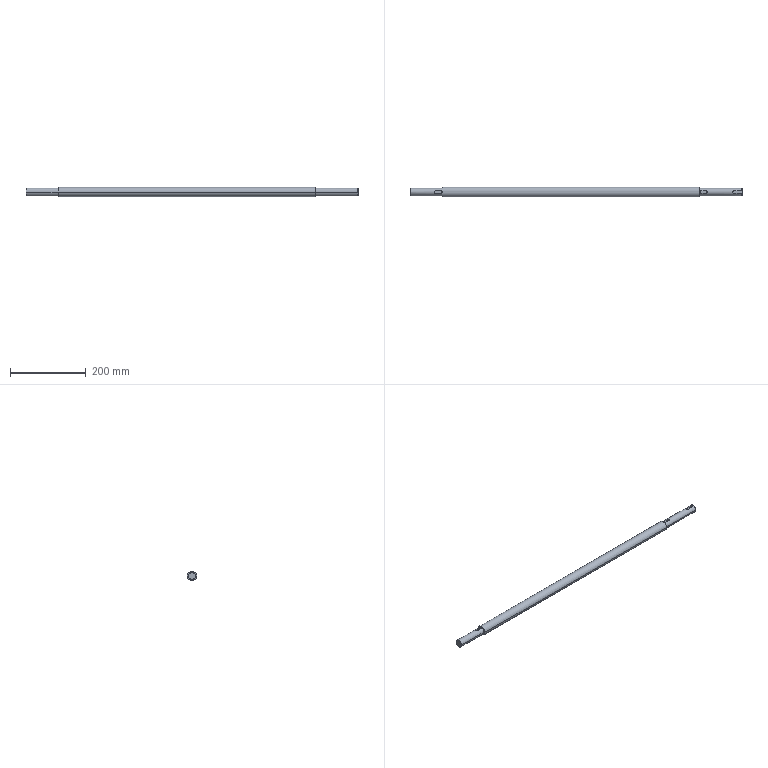Part | STEP file | J011-EBZ05-03-06-Part-1 | 1 solid | 42 faces | box 874 x 25 x 25 mm | volume 391880 mm3 | cylinder 17 | plane 14 | cone 7 | torus 4 | commonest cylinder face diameters 6 x7 20 x4 6.65 x2 8 x2 25 x2
STEP:
#1=CARTESIAN_POINT('',(852.08,0.,0.));
#2=VERTEX_POINT('',#1);
#3=CARTESIAN_POINT('',(854.,3.325,0.));
#4=VERTEX_POINT('',#3);
#5=CARTESIAN_POINT('',(854.,3.325,0.));
#6=DIRECTION('',(0.5,0.866,0.));
#7=VECTOR('',#6,1000.);
#8=LINE('',#5,#7);
#9=EDGE_CURVE('',#2,#4,#8,.T.);
#10=ORIENTED_EDGE('',*,*,#9,.F.);
#11=CARTESIAN_POINT('',(854.,-3.325,0.));
#12=VERTEX_POINT('',#11);
#13=CARTESIAN_POINT('',(854.,-3.325,0.));
#14=DIRECTION('',(0.5,-0.866,0.));
#15=VECTOR('',#14,1000.);
#16=LINE('',#13,#15);
#17=EDGE_CURVE('',#2,#12,#16,.T.);
#18=ORIENTED_EDGE('',*,*,#17,.T.);
#19=CARTESIAN_POINT('',(854.,0.,0.));
#20=DIRECTION('',(1.,0.,0.));
#21=DIRECTION('',(0.,1.,0.));
#22=AXIS2_PLACEMENT_3D('',#19,#20,#21);
#23=CIRCLE('',#22,3.325);
#24=EDGE_CURVE('',#12,#4,#23,.T.);
#25=ORIENTED_EDGE('',*,*,#24,.T.);
#26=EDGE_LOOP('',(#10,#18,#25));
#27=FACE_OUTER_BOUND('',#26,.T.);
#28=CARTESIAN_POINT('',(854.,0.,0.));
#29=DIRECTION('',(1.,0.,0.));
#30=DIRECTION('',(0.,1.,0.));
#31=AXIS2_PLACEMENT_3D('',#28,#29,#30);
#32=CONICAL_SURFACE('',#31,3.325,1.047);
#33=ADVANCED_FACE('',(#27),#32,.F.);
#34=ORIENTED_EDGE('',*,*,#24,.F.);
#35=CARTESIAN_POINT('',(858.,-3.325,0.));
#36=VERTEX_POINT('',#35);
#37=CARTESIAN_POINT('',(874.,-3.325,0.));
#38=DIRECTION('',(1.,0.,0.));
#39=VECTOR('',#38,1000.);
#40=LINE('',#37,#39);
#41=EDGE_CURVE('',#12,#36,#40,.T.);
#42=ORIENTED_EDGE('',*,*,#41,.T.);
#43=CARTESIAN_POINT('',(858.,3.325,0.));
#44=VERTEX_POINT('',#43);
#45=CARTESIAN_POINT('',(858.,0.,0.));
#46=DIRECTION('',(1.,0.,0.));
#47=DIRECTION('',(0.,1.,0.));
#48=AXIS2_PLACEMENT_3D('',#45,#46,#47);
#49=CIRCLE('',#48,3.325);
#50=EDGE_CURVE('',#36,#44,#49,.T.);
#51=ORIENTED_EDGE('',*,*,#50,.T.);
#52=CARTESIAN_POINT('',(874.,3.325,0.));
#53=DIRECTION('',(1.,0.,0.));
#54=VECTOR('',#53,1000.);
#55=LINE('',#52,#54);
#56=EDGE_CURVE('',#4,#44,#55,.T.);
#57=ORIENTED_EDGE('',*,*,#56,.F.);
#58=EDGE_LOOP('',(#34,#42,#51,#57));
#59=FACE_OUTER_BOUND('',#58,.T.);
#60=CARTESIAN_POINT('',(874.,0.,0.));
#61=DIRECTION('',(1.,0.,0.));
#62=DIRECTION('',(0.,1.,0.));
#63=AXIS2_PLACEMENT_3D('',#60,#61,#62);
#64=CYLINDRICAL_SURFACE('',#63,3.325);
#65=ADVANCED_FACE('',(#59),#64,.F.);
#66=CARTESIAN_POINT('',(858.,-4.,0.));
#67=VERTEX_POINT('',#66);
#68=CARTESIAN_POINT('',(858.,4.,0.));
#69=VERTEX_POINT('',#68);
#70=CARTESIAN_POINT('',(858.,0.,0.));
#71=DIRECTION('',(1.,0.,0.));
#72=DIRECTION('',(0.,1.,0.));
#73=AXIS2_PLACEMENT_3D('',#70,#71,#72);
#74=CIRCLE('',#73,4.);
#75=EDGE_CURVE('',#67,#69,#74,.T.);
#76=ORIENTED_EDGE('',*,*,#75,.F.);
#77=CARTESIAN_POINT('',(874.,-4.,0.));
#78=VERTEX_POINT('',#77);
#79=CARTESIAN_POINT('',(874.,-4.,0.));
#80=DIRECTION('',(1.,0.,0.));
#81=VECTOR('',#80,1000.);
#82=LINE('',#79,#81);
#83=EDGE_CURVE('',#67,#78,#82,.T.);
#84=ORIENTED_EDGE('',*,*,#83,.T.);
#85=CARTESIAN_POINT('',(874.,4.,0.));
#86=VERTEX_POINT('',#85);
#87=CARTESIAN_POINT('',(874.,0.,0.));
#88=DIRECTION('',(1.,0.,0.));
#89=DIRECTION('',(0.,1.,0.));
#90=AXIS2_PLACEMENT_3D('',#87,#88,#89);
#91=CIRCLE('',#90,4.);
#92=EDGE_CURVE('',#78,#86,#91,.T.);
#93=ORIENTED_EDGE('',*,*,#92,.T.);
#94=CARTESIAN_POINT('',(874.,4.,0.));
#95=DIRECTION('',(1.,0.,0.));
#96=VECTOR('',#95,1000.);
#97=LINE('',#94,#96);
#98=EDGE_CURVE('',#69,#86,#97,.T.);
#99=ORIENTED_EDGE('',*,*,#98,.F.);
#100=EDGE_LOOP('',(#76,#84,#93,#99));
#101=FACE_OUTER_BOUND('',#100,.T.);
#102=CARTESIAN_POINT('',(874.,0.,0.));
#103=DIRECTION('',(1.,0.,0.));
#104=DIRECTION('',(0.,1.,0.));
#105=AXIS2_PLACEMENT_3D('',#102,#103,#104);
#106=CYLINDRICAL_SURFACE('',#105,4.);
#107=ADVANCED_FACE('',(#101),#106,.F.);
#108=CARTESIAN_POINT('',(762.8,0.,10.));
#109=VERTEX_POINT('',#108);
#110=CARTESIAN_POINT('',(765.8,3.,9.539));
#111=VERTEX_POINT('',#110);
#112=CARTESIAN_POINT('',(762.8,0.,10.));
#113=CARTESIAN_POINT('',(762.8,0.1993,10.));
#114=CARTESIAN_POINT('',(762.82,0.3951,9.994));
#115=CARTESIAN_POINT('',(762.897,0.7799,9.971));
#116=CARTESIAN_POINT('',(762.955,0.971,9.954));
#117=CARTESIAN_POINT('',(763.106,1.334,9.912));
#118=CARTESIAN_POINT('',(763.198,1.505,9.887));
#119=CARTESIAN_POINT('',(763.415,1.831,9.832));
#120=CARTESIAN_POINT('',(763.541,1.984,9.802));
#121=CARTESIAN_POINT('',(763.953,2.396,9.713));
#122=CARTESIAN_POINT('',(764.286,2.619,9.652));
#123=CARTESIAN_POINT('',(764.826,2.844,9.587));
#124=CARTESIAN_POINT('',(765.016,2.902,9.57));
#125=CARTESIAN_POINT('',(765.404,2.98,9.546));
#126=CARTESIAN_POINT('',(765.601,3.,9.539));
#127=CARTESIAN_POINT('',(765.8,3.,9.539));
#128=B_SPLINE_CURVE_WITH_KNOTS('',3,(#112,#113,#114,#115,#116,#117,#118,#119,#120,#121,#122,#123,#124,#125,#126,#127),.UNSPECIFIED.,.F.,.F.,(4,2,2,2,2,2,2,4),(0.,0.0005892,0.001178,0.001768,0.002357,0.003535,0.004125,0.004714),.UNSPECIFIED.);
#129=EDGE_CURVE('',#109,#111,#128,.T.);
#130=ORIENTED_EDGE('',*,*,#129,.F.);
#131=CARTESIAN_POINT('',(762.8,0.,6.5));
#132=VERTEX_POINT('',#131);
#133=CARTESIAN_POINT('',(762.8,0.,10.52));
#134=DIRECTION('',(0.,0.,-1.));
#135=VECTOR('',#134,1000.);
#136=LINE('',#133,#135);
#137=EDGE_CURVE('',#109,#132,#136,.T.);
#138=ORIENTED_EDGE('',*,*,#137,.T.);
#139=CARTESIAN_POINT('',(765.8,3.,6.5));
#140=VERTEX_POINT('',#139);
#141=CARTESIAN_POINT('',(765.8,0.,6.5));
#142=DIRECTION('',(0.,0.,1.));
#143=DIRECTION('',(-1.,0.,0.));
#144=AXIS2_PLACEMENT_3D('',#141,#142,#143);
#145=CIRCLE('',#144,3.);
#146=EDGE_CURVE('',#140,#132,#145,.T.);
#147=ORIENTED_EDGE('',*,*,#146,.F.);
#148=CARTESIAN_POINT('',(765.8,3.,6.5));
#149=DIRECTION('',(0.,0.,-1.));
#150=VECTOR('',#149,1000.);
#151=LINE('',#148,#150);
#152=EDGE_CURVE('',#111,#140,#151,.T.);
#153=ORIENTED_EDGE('',*,*,#152,.F.);
#154=EDGE_LOOP('',(#130,#138,#147,#153));
#155=FACE_OUTER_BOUND('',#154,.T.);
#156=CARTESIAN_POINT('',(765.8,0.,10.52));
#157=DIRECTION('',(0.,0.,-1.));
#158=DIRECTION('',(-1.,0.,0.));
#159=AXIS2_PLACEMENT_3D('',#156,#157,#158);
#160=CYLINDRICAL_SURFACE('',#159,3.);
#161=ADVANCED_FACE('',(#155),#160,.F.);
#162=CARTESIAN_POINT('',(64.15,0.,10.));
#163=VERTEX_POINT('',#162);
#164=CARTESIAN_POINT('',(67.15,3.,9.539));
#165=VERTEX_POINT('',#164);
#166=CARTESIAN_POINT('',(64.15,0.,10.));
#167=CARTESIAN_POINT('',(64.15,0.1968,10.));
#168=CARTESIAN_POINT('',(64.17,0.3967,9.994));
#169=CARTESIAN_POINT('',(64.247,0.7821,9.971));
#170=CARTESIAN_POINT('',(64.304,0.9695,9.955));
#171=CARTESIAN_POINT('',(64.456,1.334,9.912));
#172=CARTESIAN_POINT('',(64.549,1.507,9.887));
#173=CARTESIAN_POINT('',(64.766,1.831,9.832));
#174=CARTESIAN_POINT('',(64.891,1.983,9.802));
#175=CARTESIAN_POINT('',(65.167,2.26,9.742));
#176=CARTESIAN_POINT('',(65.317,2.383,9.713));
#177=CARTESIAN_POINT('',(65.641,2.6,9.657));
#178=CARTESIAN_POINT('',(65.817,2.694,9.63));
#179=CARTESIAN_POINT('',(66.178,2.845,9.587));
#180=CARTESIAN_POINT('',(66.365,2.902,9.57));
#181=CARTESIAN_POINT('',(66.751,2.98,9.546));
#182=CARTESIAN_POINT('',(66.951,3.,9.539));
#183=CARTESIAN_POINT('',(67.15,3.,9.539));
#184=B_SPLINE_CURVE_WITH_KNOTS('',3,(#166,#167,#168,#169,#170,#171,#172,#173,#174,#175,#176,#177,#178,#179,#180,#181,#182,#183),.UNSPECIFIED.,.F.,.F.,(4,2,2,2,2,2,2,2,4),(0.004718,0.005307,0.005896,0.006485,0.007074,0.007663,0.008252,0.008842,0.009431),.UNSPECIFIED.);
#185=EDGE_CURVE('',#163,#165,#184,.T.);
#186=ORIENTED_EDGE('',*,*,#185,.F.);
#187=CARTESIAN_POINT('',(64.15,0.,6.5));
#188=VERTEX_POINT('',#187);
#189=CARTESIAN_POINT('',(64.15,0.,10.));
#190=DIRECTION('',(0.,0.,-1.));
#191=VECTOR('',#190,1000.);
#192=LINE('',#189,#191);
#193=EDGE_CURVE('',#163,#188,#192,.T.);
#194=ORIENTED_EDGE('',*,*,#193,.T.);
#195=CARTESIAN_POINT('',(67.15,3.,6.5));
#196=VERTEX_POINT('',#195);
#197=CARTESIAN_POINT('',(67.15,0.,6.5));
#198=DIRECTION('',(0.,0.,1.));
#199=DIRECTION('',(1.,0.,0.));
#200=AXIS2_PLACEMENT_3D('',#197,#198,#199);
#201=CIRCLE('',#200,3.);
#202=EDGE_CURVE('',#196,#188,#201,.T.);
#203=ORIENTED_EDGE('',*,*,#202,.F.);
#204=CARTESIAN_POINT('',(67.15,3.,10.));
#205=DIRECTION('',(0.,0.,-1.));
#206=VECTOR('',#205,1000.);
#207=LINE('',#204,#206);
#208=EDGE_CURVE('',#165,#196,#207,.T.);
#209=ORIENTED_EDGE('',*,*,#208,.F.);
#210=EDGE_LOOP('',(#186,#194,#203,#209));
#211=FACE_OUTER_BOUND('',#210,.T.);
#212=CARTESIAN_POINT('',(67.15,0.,10.));
#213=DIRECTION('',(0.,0.,-1.));
#214=DIRECTION('',(-1.,0.,0.));
#215=AXIS2_PLACEMENT_3D('',#212,#213,#214);
#216=CYLINDRICAL_SURFACE('',#215,3.);
#217=ADVANCED_FACE('',(#211),#216,.F.);
#218=CARTESIAN_POINT('',(762.3,10.,0.));
#219=VERTEX_POINT('',#218);
#220=CARTESIAN_POINT('',(762.3,-10.,0.));
#221=VERTEX_POINT('',#220);
#222=CARTESIAN_POINT('',(762.3,0.,0.));
#223=DIRECTION('',(1.,0.,0.));
#224=DIRECTION('',(0.,-1.,0.));
#225=AXIS2_PLACEMENT_3D('',#222,#223,#224);
#226=CIRCLE('',#225,10.);
#227=EDGE_CURVE('',#219,#221,#226,.T.);
#228=ORIENTED_EDGE('',*,*,#227,.F.);
#229=CARTESIAN_POINT('',(761.8,10.5,0.));
#230=VERTEX_POINT('',#229);
#231=CARTESIAN_POINT('',(762.3,10.5,0.));
#232=DIRECTION('',(0.,0.,-1.));
#233=DIRECTION('',(0.,1.,0.));
#234=AXIS2_PLACEMENT_3D('',#231,#232,#233);
#235=CIRCLE('',#234,0.5);
#236=EDGE_CURVE('',#219,#230,#235,.T.);
#237=ORIENTED_EDGE('',*,*,#236,.T.);
#238=CARTESIAN_POINT('',(761.8,-10.5,0.));
#239=VERTEX_POINT('',#238);
#240=CARTESIAN_POINT('',(761.8,0.,0.));
#241=DIRECTION('',(-1.,0.,0.));
#242=DIRECTION('',(0.,-1.,0.));
#243=AXIS2_PLACEMENT_3D('',#240,#241,#242);
#244=CIRCLE('',#243,10.5);
#245=EDGE_CURVE('',#239,#230,#244,.T.);
#246=ORIENTED_EDGE('',*,*,#245,.F.);
#247=CARTESIAN_POINT('',(762.3,-10.5,0.));
#248=DIRECTION('',(0.,0.,1.));
#249=DIRECTION('',(1.,0.,0.));
#250=AXIS2_PLACEMENT_3D('',#247,#248,#249);
#251=CIRCLE('',#250,0.5);
#252=EDGE_CURVE('',#221,#239,#251,.T.);
#253=ORIENTED_EDGE('',*,*,#252,.F.);
#254=EDGE_LOOP('',(#228,#237,#246,#253));
#255=FACE_OUTER_BOUND('',#254,.T.);
#256=CARTESIAN_POINT('',(762.3,0.,0.));
#257=DIRECTION('',(1.,0.,0.));
#258=DIRECTION('',(0.,-1.,0.));
#259=AXIS2_PLACEMENT_3D('',#256,#257,#258);
#260=TOROIDAL_SURFACE('',#259,10.5,0.5);
#261=ADVANCED_FACE('',(#255),#260,.F.);
#262=CARTESIAN_POINT('',(84.7,-10.,0.));
#263=VERTEX_POINT('',#262);
#264=CARTESIAN_POINT('',(84.7,10.,0.));
#265=VERTEX_POINT('',#264);
#266=CARTESIAN_POINT('',(84.7,0.,0.));
#267=DIRECTION('',(-1.,0.,0.));
#268=DIRECTION('',(0.,1.,0.));
#269=AXIS2_PLACEMENT_3D('',#266,#267,#268);
#270=CIRCLE('',#269,10.);
#271=EDGE_CURVE('',#263,#265,#270,.T.);
#272=ORIENTED_EDGE('',*,*,#271,.F.);
#273=CARTESIAN_POINT('',(85.2,-10.5,0.));
#274=VERTEX_POINT('',#273);
#275=CARTESIAN_POINT('',(84.7,-10.5,0.));
#276=DIRECTION('',(0.,0.,-1.));
#277=DIRECTION('',(0.,1.,0.));
#278=AXIS2_PLACEMENT_3D('',#275,#276,#277);
#279=CIRCLE('',#278,0.5);
#280=EDGE_CURVE('',#263,#274,#279,.T.);
#281=ORIENTED_EDGE('',*,*,#280,.T.);
#282=CARTESIAN_POINT('',(85.2,10.5,0.));
#283=VERTEX_POINT('',#282);
#284=CARTESIAN_POINT('',(85.2,0.,0.));
#285=DIRECTION('',(1.,0.,0.));
#286=DIRECTION('',(0.,1.,0.));
#287=AXIS2_PLACEMENT_3D('',#284,#285,#286);
#288=CIRCLE('',#287,10.5);
#289=EDGE_CURVE('',#283,#274,#288,.T.);
#290=ORIENTED_EDGE('',*,*,#289,.F.);
#291=CARTESIAN_POINT('',(84.7,10.5,0.));
#292=DIRECTION('',(0.,0.,1.));
#293=DIRECTION('',(1.,0.,0.));
#294=AXIS2_PLACEMENT_3D('',#291,#292,#293);
#295=CIRCLE('',#294,0.5);
#296=EDGE_CURVE('',#265,#283,#295,.T.);
#297=ORIENTED_EDGE('',*,*,#296,.F.);
#298=EDGE_LOOP('',(#272,#281,#290,#297));
#299=FACE_OUTER_BOUND('',#298,.T.);
#300=CARTESIAN_POINT('',(84.7,0.,0.));
#301=DIRECTION('',(-1.,0.,0.));
#302=DIRECTION('',(0.,1.,0.));
#303=AXIS2_PLACEMENT_3D('',#300,#301,#302);
#304=TOROIDAL_SURFACE('',#303,10.5,0.5);
#305=ADVANCED_FACE('',(#299),#304,.F.);
#306=CARTESIAN_POINT('',(0.,-9.,0.));
#307=VERTEX_POINT('',#306);
#308=CARTESIAN_POINT('',(0.,9.,0.));
#309=VERTEX_POINT('',#308);
#310=CARTESIAN_POINT('',(0.,0.,0.));
#311=DIRECTION('',(1.,0.,0.));
#312=DIRECTION('',(0.,-1.,0.));
#313=AXIS2_PLACEMENT_3D('',#310,#311,#312);
#314=CIRCLE('',#313,9.);
#315=EDGE_CURVE('',#307,#309,#314,.T.);
#316=ORIENTED_EDGE('',*,*,#315,.T.);
#317=CARTESIAN_POINT('',(1.,10.,0.));
#318=VERTEX_POINT('',#317);
#319=CARTESIAN_POINT('',(1.,10.,0.));
#320=DIRECTION('',(0.7071,0.7071,0.));
#321=VECTOR('',#320,1000.);
#322=LINE('',#319,#321);
#323=EDGE_CURVE('',#309,#318,#322,.T.);
#324=ORIENTED_EDGE('',*,*,#323,.T.);
#325=CARTESIAN_POINT('',(1.,-10.,0.));
#326=VERTEX_POINT('',#325);
#327=CARTESIAN_POINT('',(1.,0.,0.));
#328=DIRECTION('',(1.,0.,0.));
#329=DIRECTION('',(0.,-1.,0.));
#330=AXIS2_PLACEMENT_3D('',#327,#328,#329);
#331=CIRCLE('',#330,10.);
#332=EDGE_CURVE('',#326,#318,#331,.T.);
#333=ORIENTED_EDGE('',*,*,#332,.F.);
#334=CARTESIAN_POINT('',(1.,-10.,0.));
#335=DIRECTION('',(0.7071,-0.7071,0.));
#336=VECTOR('',#335,1000.);
#337=LINE('',#334,#336);
#338=EDGE_CURVE('',#307,#326,#337,.T.);
#339=ORIENTED_EDGE('',*,*,#338,.F.);
#340=EDGE_LOOP('',(#316,#324,#333,#339));
#341=FACE_OUTER_BOUND('',#340,.T.);
#342=CARTESIAN_POINT('',(1.,0.,0.));
#343=DIRECTION('',(1.,0.,0.));
#344=DIRECTION('',(0.,-1.,0.));
#345=AXIS2_PLACEMENT_3D('',#342,#343,#344);
#346=CONICAL_SURFACE('',#345,10.,0.7854);
#347=ADVANCED_FACE('',(#341),#346,.T.);
#348=CARTESIAN_POINT('',(85.2,-12.5,0.));
#349=VERTEX_POINT('',#348);
#350=CARTESIAN_POINT('',(85.2,12.5,0.));
#351=VERTEX_POINT('',#350);
#352=CARTESIAN_POINT('',(85.2,0.,0.));
#353=DIRECTION('',(1.,0.,0.));
#354=DIRECTION('',(0.,-1.,0.));
#355=AXIS2_PLACEMENT_3D('',#352,#353,#354);
#356=CIRCLE('',#355,12.5);
#357=EDGE_CURVE('',#349,#351,#356,.T.);
#358=ORIENTED_EDGE('',*,*,#357,.T.);
#359=CARTESIAN_POINT('',(761.8,12.5,0.));
#360=VERTEX_POINT('',#359);
#361=CARTESIAN_POINT('',(154.523,12.5,0.));
#362=DIRECTION('',(1.,0.,0.));
#363=VECTOR('',#362,1000.);
#364=LINE('',#361,#363);
#365=EDGE_CURVE('',#351,#360,#364,.T.);
#366=ORIENTED_EDGE('',*,*,#365,.T.);
#367=CARTESIAN_POINT('',(761.8,-12.5,0.));
#368=VERTEX_POINT('',#367);
#369=CARTESIAN_POINT('',(761.8,0.,0.));
#370=DIRECTION('',(1.,0.,0.));
#371=DIRECTION('',(0.,-1.,0.));
#372=AXIS2_PLACEMENT_3D('',#369,#370,#371);
#373=CIRCLE('',#372,12.5);
#374=EDGE_CURVE('',#368,#360,#373,.T.);
#375=ORIENTED_EDGE('',*,*,#374,.F.);
#376=CARTESIAN_POINT('',(154.523,-12.5,0.));
#377=DIRECTION('',(1.,0.,0.));
#378=VECTOR('',#377,1000.);
#379=LINE('',#376,#378);
#380=EDGE_CURVE('',#349,#368,#379,.T.);
#381=ORIENTED_EDGE('',*,*,#380,.F.);
#382=EDGE_LOOP('',(#358,#366,#375,#381));
#383=FACE_OUTER_BOUND('',#382,.T.);
#384=CARTESIAN_POINT('',(154.523,0.,0.));
#385=DIRECTION('',(1.,0.,0.));
#386=DIRECTION('',(0.,-1.,0.));
#387=AXIS2_PLACEMENT_3D('',#384,#385,#386);
#388=CYLINDRICAL_SURFACE('',#387,12.5);
#389=ADVANCED_FACE('',(#383),#388,.T.);
#390=CARTESIAN_POINT('',(762.3,0.,0.));
#391=DIRECTION('',(1.,0.,0.));
#392=DIRECTION('',(0.,-1.,0.));
#393=AXIS2_PLACEMENT_3D('',#390,#391,#392);
#394=CIRCLE('',#393,10.);
#395=EDGE_CURVE('',#221,#219,#394,.T.);
#396=ORIENTED_EDGE('',*,*,#395,.T.);
#397=CARTESIAN_POINT('',(873.,10.,0.));
#398=VERTEX_POINT('',#397);
#399=CARTESIAN_POINT('',(154.523,10.,0.));
#400=DIRECTION('',(1.,0.,0.));
#401=VECTOR('',#400,1000.);
#402=LINE('',#399,#401);
#403=EDGE_CURVE('',#219,#398,#402,.T.);
#404=ORIENTED_EDGE('',*,*,#403,.T.);
#405=CARTESIAN_POINT('',(873.,-10.,0.));
#406=VERTEX_POINT('',#405);
#407=CARTESIAN_POINT('',(873.,0.,0.));
#408=DIRECTION('',(1.,0.,0.));
#409=DIRECTION('',(0.,-1.,0.));
#410=AXIS2_PLACEMENT_3D('',#407,#408,#409);
#411=CIRCLE('',#410,10.);
#412=EDGE_CURVE('',#406,#398,#411,.T.);
#413=ORIENTED_EDGE('',*,*,#412,.F.);
#414=CARTESIAN_POINT('',(154.523,-10.,0.));
#415=DIRECTION('',(1.,0.,0.));
#416=VECTOR('',#415,1000.);
#417=LINE('',#414,#416);
#418=EDGE_CURVE('',#221,#406,#417,.T.);
#419=ORIENTED_EDGE('',*,*,#418,.F.);
#420=EDGE_LOOP('',(#396,#404,#413,#419));
#421=FACE_OUTER_BOUND('',#420,.T.);
#422=CARTESIAN_POINT('',(154.523,0.,0.));
#423=DIRECTION('',(1.,0.,0.));
#424=DIRECTION('',(0.,-1.,0.));
#425=AXIS2_PLACEMENT_3D('',#422,#423,#424);
#426=CYLINDRICAL_SURFACE('',#425,10.);
#427=ADVANCED_FACE('',(#421),#426,.T.);
#428=CARTESIAN_POINT('',(874.,-9.,0.));
#429=VERTEX_POINT('',#428);
#430=CARTESIAN_POINT('',(874.,9.,0.));
#431=VERTEX_POINT('',#430);
#432=CARTESIAN_POINT('',(874.,0.,0.));
#433=DIRECTION('',(1.,0.,0.));
#434=DIRECTION('',(0.,-1.,0.));
#435=AXIS2_PLACEMENT_3D('',#432,#433,#434);
#436=CIRCLE('',#435,9.);
#437=EDGE_CURVE('',#429,#431,#436,.T.);
#438=ORIENTED_EDGE('',*,*,#437,.F.);
#439=CARTESIAN_POINT('',(874.,-9.,0.));
#440=DIRECTION('',(-0.7071,-0.7071,0.));
#441=VECTOR('',#440,1000.);
#442=LINE('',#439,#441);
#443=EDGE_CURVE('',#429,#406,#442,.T.);
#444=ORIENTED_EDGE('',*,*,#443,.T.);
#445=ORIENTED_EDGE('',*,*,#412,.T.);
#446=CARTESIAN_POINT('',(874.,9.,0.));
#447=DIRECTION('',(-0.7071,0.7071,0.));
#448=VECTOR('',#447,1000.);
#449=LINE('',#446,#448);
#450=EDGE_CURVE('',#431,#398,#449,.T.);
#451=ORIENTED_EDGE('',*,*,#450,.F.);
#452=EDGE_LOOP('',(#438,#444,#445,#451));
#453=FACE_OUTER_BOUND('',#452,.T.);
#454=CARTESIAN_POINT('',(874.,0.,0.));
#455=DIRECTION('',(-1.,0.,0.));
#456=DIRECTION('',(0.,1.,0.));
#457=AXIS2_PLACEMENT_3D('',#454,#455,#456);
#458=CONICAL_SURFACE('',#457,9.,0.7854);
#459=ADVANCED_FACE('',(#453),#458,.T.);
#460=CARTESIAN_POINT('',(874.,3.,8.485));
#461=VERTEX_POINT('',#460);
#462=CARTESIAN_POINT('',(874.,0.,0.));
#463=DIRECTION('',(1.,0.,0.));
#464=DIRECTION('',(0.,-1.,0.));
#465=AXIS2_PLACEMENT_3D('',#462,#463,#464);
#466=CIRCLE('',#465,9.);
#467=EDGE_CURVE('',#431,#461,#466,.T.);
#468=ORIENTED_EDGE('',*,*,#467,.F.);
#469=ORIENTED_EDGE('',*,*,#450,.T.);
#470=CARTESIAN_POINT('',(873.,3.,9.539));
#471=VERTEX_POINT('',#470);
#472=CARTESIAN_POINT('',(873.,0.,0.));
#473=DIRECTION('',(1.,0.,0.));
#474=DIRECTION('',(0.,-1.,0.));
#475=AXIS2_PLACEMENT_3D('',#472,#473,#474);
#476=CIRCLE('',#475,10.);
#477=EDGE_CURVE('',#398,#471,#476,.T.);
#478=ORIENTED_EDGE('',*,*,#477,.T.);
#479=CARTESIAN_POINT('',(874.,3.,8.485));
#480=CARTESIAN_POINT('',(873.668,3.,8.838));
#481=CARTESIAN_POINT('',(873.334,3.,9.189));
#482=CARTESIAN_POINT('',(873.,3.,9.539));
#483=B_SPLINE_CURVE_WITH_KNOTS('',3,(#479,#480,#481,#482),.UNSPECIFIED.,.F.,.F.,(4,4),(0.005441,0.006894),.UNSPECIFIED.);
#484=EDGE_CURVE('',#461,#471,#483,.T.);
#485=ORIENTED_EDGE('',*,*,#484,.F.);
#486=EDGE_LOOP('',(#468,#469,#478,#485));
#487=FACE_OUTER_BOUND('',#486,.T.);
#488=CARTESIAN_POINT('',(874.,0.,0.));
#489=DIRECTION('',(-1.,0.,0.));
#490=DIRECTION('',(0.,1.,0.));
#491=AXIS2_PLACEMENT_3D('',#488,#489,#490);
#492=CONICAL_SURFACE('',#491,9.,0.7854);
#493=ADVANCED_FACE('',(#487),#492,.T.);
#494=ORIENTED_EDGE('',*,*,#332,.T.);
#495=CARTESIAN_POINT('',(154.523,10.,0.));
#496=DIRECTION('',(1.,0.,0.));
#497=VECTOR('',#496,1000.);
#498=LINE('',#495,#497);
#499=EDGE_CURVE('',#318,#265,#498,.T.);
#500=ORIENTED_EDGE('',*,*,#499,.T.);
#501=CARTESIAN_POINT('',(84.7,0.,0.));
#502=DIRECTION('',(-1.,0.,0.));
#503=DIRECTION('',(0.,1.,0.));
#504=AXIS2_PLACEMENT_3D('',#501,#502,#503);
#505=CIRCLE('',#504,10.);
#506=EDGE_CURVE('',#265,#263,#505,.T.);
#507=ORIENTED_EDGE('',*,*,#506,.T.);
#508=CARTESIAN_POINT('',(154.523,-10.,0.));
#509=DIRECTION('',(1.,0.,0.));
#510=VECTOR('',#509,1000.);
#511=LINE('',#508,#510);
#512=EDGE_CURVE('',#326,#263,#511,.T.);
#513=ORIENTED_EDGE('',*,*,#512,.F.);
#514=EDGE_LOOP('',(#494,#500,#507,#513));
#515=FACE_OUTER_BOUND('',#514,.T.);
#516=CARTESIAN_POINT('',(154.523,0.,0.));
#517=DIRECTION('',(1.,0.,0.));
#518=DIRECTION('',(0.,-1.,0.));
#519=AXIS2_PLACEMENT_3D('',#516,#517,#518);
#520=CYLINDRICAL_SURFACE('',#519,10.);
#521=ADVANCED_FACE('',(#515),#520,.T.);
#522=CARTESIAN_POINT('',(874.,0.,0.));
#523=DIRECTION('',(1.,0.,0.));
#524=DIRECTION('',(0.,1.,0.));
#525=AXIS2_PLACEMENT_3D('',#522,#523,#524);
#526=CIRCLE('',#525,4.);
#527=EDGE_CURVE('',#86,#78,#526,.T.);
#528=ORIENTED_EDGE('',*,*,#527,.F.);
#529=ORIENTED_EDGE('',*,*,#92,.F.);
#530=EDGE_LOOP('',(#528,#529));
#531=FACE_BOUND('',#530,.T.);
#532=CARTESIAN_POINT('',(874.,3.,6.5));
#533=VERTEX_POINT('',#532);
#534=CARTESIAN_POINT('',(874.,-3.,6.5));
#535=VERTEX_POINT('',#534);
#536=CARTESIAN_POINT('',(874.,0.,6.5));
#537=DIRECTION('',(0.,-1.,0.));
#538=VECTOR('',#537,1000.);
#539=LINE('',#536,#538);
#540=EDGE_CURVE('',#533,#535,#539,.T.);
#541=ORIENTED_EDGE('',*,*,#540,.T.);
#542=CARTESIAN_POINT('',(874.,-3.,8.485));
#543=VERTEX_POINT('',#542);
#544=CARTESIAN_POINT('',(874.,-3.,10.52));
#545=DIRECTION('',(0.,0.,1.));
#546=VECTOR('',#545,1000.);
#547=LINE('',#544,#546);
#548=EDGE_CURVE('',#535,#543,#547,.T.);
#549=ORIENTED_EDGE('',*,*,#548,.T.);
#550=CARTESIAN_POINT('',(874.,0.,0.));
#551=DIRECTION('',(1.,0.,0.));
#552=DIRECTION('',(0.,-1.,0.));
#553=AXIS2_PLACEMENT_3D('',#550,#551,#552);
#554=CIRCLE('',#553,9.);
#555=EDGE_CURVE('',#543,#429,#554,.T.);
#556=ORIENTED_EDGE('',*,*,#555,.T.);
#557=ORIENTED_EDGE('',*,*,#437,.T.);
#558=ORIENTED_EDGE('',*,*,#467,.T.);
#559=CARTESIAN_POINT('',(874.,3.,10.52));
#560=DIRECTION('',(0.,0.,-1.));
#561=VECTOR('',#560,1000.);
#562=LINE('',#559,#561);
#563=EDGE_CURVE('',#461,#533,#562,.T.);
#564=ORIENTED_EDGE('',*,*,#563,.T.);
#565=EDGE_LOOP('',(#541,#549,#556,#557,#558,#564));
#566=FACE_OUTER_BOUND('',#565,.T.);
#567=CARTESIAN_POINT('',(874.,0.,0.));
#568=DIRECTION('',(1.,0.,0.));
#569=DIRECTION('',(0.,-1.,0.));
#570=AXIS2_PLACEMENT_3D('',#567,#568,#569);
#571=PLANE('',#570);
#572=ADVANCED_FACE('',(#531,#566),#571,.T.);
#573=ORIENTED_EDGE('',*,*,#499,.F.);
#574=CARTESIAN_POINT('',(1.,0.,0.));
#575=DIRECTION('',(1.,0.,0.));
#576=DIRECTION('',(0.,-1.,0.));
#577=AXIS2_PLACEMENT_3D('',#574,#575,#576);
#578=CIRCLE('',#577,10.);
#579=EDGE_CURVE('',#318,#326,#578,.T.);
#580=ORIENTED_EDGE('',*,*,#579,.T.);
#581=ORIENTED_EDGE('',*,*,#512,.T.);
#582=ORIENTED_EDGE('',*,*,#271,.T.);
#583=EDGE_LOOP('',(#573,#580,#581,#582));
#584=FACE_OUTER_BOUND('',#583,.T.);
#585=CARTESIAN_POINT('',(81.15,3.,9.539));
#586=VERTEX_POINT('',#585);
#587=CARTESIAN_POINT('',(154.523,3.,9.539));
#588=DIRECTION('',(1.,0.,0.));
#589=VECTOR('',#588,1000.);
#590=LINE('',#587,#589);
#591=EDGE_CURVE('',#165,#586,#590,.T.);
#592=ORIENTED_EDGE('',*,*,#591,.T.);
#593=CARTESIAN_POINT('',(81.15,-3.,9.539));
#594=VERTEX_POINT('',#593);
#595=CARTESIAN_POINT('',(81.15,3.,9.539));
#596=CARTESIAN_POINT('',(81.349,3.,9.539));
#597=CARTESIAN_POINT('',(81.545,2.98,9.546));
#598=CARTESIAN_POINT('',(81.93,2.903,9.569));
#599=CARTESIAN_POINT('',(82.121,2.845,9.587));
#600=CARTESIAN_POINT('',(82.484,2.694,9.631));
#601=CARTESIAN_POINT('',(82.656,2.602,9.656));
#602=CARTESIAN_POINT('',(82.981,2.385,9.712));
#603=CARTESIAN_POINT('',(83.134,2.259,9.743));
#604=CARTESIAN_POINT('',(83.546,1.847,9.832));
#605=CARTESIAN_POINT('',(83.769,1.514,9.891));
#606=CARTESIAN_POINT('',(83.994,0.9732,9.954));
#607=CARTESIAN_POINT('',(84.053,0.783,9.971));
#608=CARTESIAN_POINT('',(84.13,0.3953,9.994));
#609=CARTESIAN_POINT('',(84.15,0.1999,10.));
#610=CARTESIAN_POINT('',(84.15,-0.194,10.));
#611=CARTESIAN_POINT('',(84.131,-0.394,9.994));
#612=CARTESIAN_POINT('',(84.054,-0.7797,9.971));
#613=CARTESIAN_POINT('',(83.997,-0.9673,9.955));
#614=CARTESIAN_POINT('',(83.845,-1.332,9.913));
#615=CARTESIAN_POINT('',(83.752,-1.506,9.887));
#616=CARTESIAN_POINT('',(83.536,-1.83,9.833));
#617=CARTESIAN_POINT('',(83.41,-1.982,9.803));
#618=CARTESIAN_POINT('',(83.134,-2.259,9.743));
#619=CARTESIAN_POINT('',(82.983,-2.383,9.713));
#620=CARTESIAN_POINT('',(82.66,-2.6,9.657));
#621=CARTESIAN_POINT('',(82.484,-2.694,9.631));
#622=CARTESIAN_POINT('',(82.123,-2.845,9.587));
#623=CARTESIAN_POINT('',(81.936,-2.902,9.57));
#624=CARTESIAN_POINT('',(81.549,-2.98,9.546));
#625=CARTESIAN_POINT('',(81.349,-3.,9.539));
#626=CARTESIAN_POINT('',(81.15,-3.,9.539));
#627=B_SPLINE_CURVE_WITH_KNOTS('',3,(#595,#596,#597,#598,#599,#600,#601,#602,#603,#604,#605,#606,#607,#608,#609,#610,#611,#612,#613,#614,#615,#616,#617,#618,#619,#620,#621,#622,#623,#624,#625,#626),.UNSPECIFIED.,.F.,.F.,(4,2,2,2,2,2,2,2,2,2,2,2,2,2,2,4),(0.,0.0005894,0.001179,0.001768,0.002358,0.003536,0.004126,0.004715,0.005305,0.005894,0.006484,0.007073,0.007662,0.008252,0.008841,0.009431),.UNSPECIFIED.);
#628=EDGE_CURVE('',#586,#594,#627,.T.);
#629=ORIENTED_EDGE('',*,*,#628,.T.);
#630=CARTESIAN_POINT('',(67.15,-3.,9.539));
#631=VERTEX_POINT('',#630);
#632=CARTESIAN_POINT('',(154.523,-3.,9.539));
#633=DIRECTION('',(-1.,0.,0.));
#634=VECTOR('',#633,1000.);
#635=LINE('',#632,#634);
#636=EDGE_CURVE('',#594,#631,#635,.T.);
#637=ORIENTED_EDGE('',*,*,#636,.T.);
#638=CARTESIAN_POINT('',(67.15,-3.,9.539));
#639=CARTESIAN_POINT('',(66.95,-3.,9.539));
#640=CARTESIAN_POINT('',(66.755,-2.98,9.546));
#641=CARTESIAN_POINT('',(66.369,-2.903,9.569));
#642=CARTESIAN_POINT('',(66.178,-2.845,9.587));
#643=CARTESIAN_POINT('',(65.815,-2.694,9.631));
#644=CARTESIAN_POINT('',(65.644,-2.602,9.656));
#645=CARTESIAN_POINT('',(65.318,-2.384,9.712));
#646=CARTESIAN_POINT('',(65.165,-2.258,9.743));
#647=CARTESIAN_POINT('',(64.753,-1.845,9.832));
#648=CARTESIAN_POINT('',(64.53,-1.512,9.892));
#649=CARTESIAN_POINT('',(64.305,-0.971,9.954));
#650=CARTESIAN_POINT('',(64.247,-0.7806,9.971));
#651=CARTESIAN_POINT('',(64.169,-0.3926,9.994));
#652=CARTESIAN_POINT('',(64.15,-0.197,10.));
#653=CARTESIAN_POINT('',(64.15,0.,10.));
#654=B_SPLINE_CURVE_WITH_KNOTS('',3,(#638,#639,#640,#641,#642,#643,#644,#645,#646,#647,#648,#649,#650,#651,#652,#653),.UNSPECIFIED.,.F.,.F.,(4,2,2,2,2,2,2,4),(0.,0.0005898,0.00118,0.001769,0.002359,0.003539,0.004128,0.004718),.UNSPECIFIED.);
#655=EDGE_CURVE('',#631,#163,#654,.T.);
#656=ORIENTED_EDGE('',*,*,#655,.T.);
#657=ORIENTED_EDGE('',*,*,#185,.T.);
#658=EDGE_LOOP('',(#592,#629,#637,#656,#657));
#659=FACE_BOUND('',#658,.T.);
#660=CARTESIAN_POINT('',(154.523,0.,0.));
#661=DIRECTION('',(1.,0.,0.));
#662=DIRECTION('',(0.,-1.,0.));
#663=AXIS2_PLACEMENT_3D('',#660,#661,#662);
#664=CYLINDRICAL_SURFACE('',#663,10.);
#665=ADVANCED_FACE('',(#584,#659),#664,.T.);
#666=ORIENTED_EDGE('',*,*,#443,.F.);
#667=ORIENTED_EDGE('',*,*,#555,.F.);
#668=CARTESIAN_POINT('',(873.,-3.,9.539));
#669=VERTEX_POINT('',#668);
#670=CARTESIAN_POINT('',(873.,-3.,9.539));
#671=CARTESIAN_POINT('',(873.334,-3.,9.189));
#672=CARTESIAN_POINT('',(873.668,-3.,8.838));
#673=CARTESIAN_POINT('',(874.,-3.,8.485));
#674=B_SPLINE_CURVE_WITH_KNOTS('',3,(#670,#671,#672,#673),.UNSPECIFIED.,.F.,.F.,(4,4),(0.005238,0.006691),.UNSPECIFIED.);
#675=EDGE_CURVE('',#669,#543,#674,.T.);
#676=ORIENTED_EDGE('',*,*,#675,.F.);
#677=CARTESIAN_POINT('',(873.,0.,0.));
#678=DIRECTION('',(1.,0.,0.));
#679=DIRECTION('',(0.,-1.,0.));
#680=AXIS2_PLACEMENT_3D('',#677,#678,#679);
#681=CIRCLE('',#680,10.);
#682=EDGE_CURVE('',#669,#406,#681,.T.);
#683=ORIENTED_EDGE('',*,*,#682,.T.);
#684=EDGE_LOOP('',(#666,#667,#676,#683));
#685=FACE_OUTER_BOUND('',#684,.T.);
#686=CARTESIAN_POINT('',(874.,0.,0.));
#687=DIRECTION('',(-1.,0.,0.));
#688=DIRECTION('',(0.,1.,0.));
#689=AXIS2_PLACEMENT_3D('',#686,#687,#688);
#690=CONICAL_SURFACE('',#689,9.,0.7854);
#691=ADVANCED_FACE('',(#685),#690,.T.);
#692=ORIENTED_EDGE('',*,*,#403,.F.);
#693=ORIENTED_EDGE('',*,*,#227,.T.);
#694=ORIENTED_EDGE('',*,*,#418,.T.);
#695=ORIENTED_EDGE('',*,*,#682,.F.);
#696=CARTESIAN_POINT('',(852.,-3.,9.539));
#697=VERTEX_POINT('',#696);
#698=CARTESIAN_POINT('',(154.523,-3.,9.539));
#699=DIRECTION('',(1.,0.,0.));
#700=VECTOR('',#699,1000.);
#701=LINE('',#698,#700);
#702=EDGE_CURVE('',#697,#669,#701,.T.);
#703=ORIENTED_EDGE('',*,*,#702,.F.);
#704=CARTESIAN_POINT('',(852.,3.,9.539));
#705=VERTEX_POINT('',#704);
#706=CARTESIAN_POINT('',(852.,-3.,9.539));
#707=CARTESIAN_POINT('',(851.801,-3.,9.539));
#708=CARTESIAN_POINT('',(851.605,-2.98,9.546));
#709=CARTESIAN_POINT('',(851.22,-2.904,9.569));
#710=CARTESIAN_POINT('',(851.029,-2.845,9.587));
#711=CARTESIAN_POINT('',(850.667,-2.695,9.63));
#712=CARTESIAN_POINT('',(850.495,-2.602,9.656));
#713=CARTESIAN_POINT('',(850.17,-2.385,9.712));
#714=CARTESIAN_POINT('',(850.017,-2.259,9.742));
#715=CARTESIAN_POINT('',(849.604,-1.847,9.832));
#716=CARTESIAN_POINT('',(849.381,-1.515,9.891));
#717=CARTESIAN_POINT('',(849.156,-0.9743,9.954));
#718=CARTESIAN_POINT('',(849.098,-0.7844,9.971));
#719=CARTESIAN_POINT('',(849.02,-0.396,9.994));
#720=CARTESIAN_POINT('',(849.,-0.1993,10.));
#721=CARTESIAN_POINT('',(849.,0.1994,10.));
#722=CARTESIAN_POINT('',(849.02,0.3951,9.994));
#723=CARTESIAN_POINT('',(849.097,0.7799,9.971));
#724=CARTESIAN_POINT('',(849.155,0.971,9.954));
#725=CARTESIAN_POINT('',(849.306,1.334,9.912));
#726=CARTESIAN_POINT('',(849.398,1.505,9.887));
#727=CARTESIAN_POINT('',(849.615,1.831,9.832));
#728=CARTESIAN_POINT('',(849.741,1.984,9.802));
#729=CARTESIAN_POINT('',(850.153,2.396,9.713));
#730=CARTESIAN_POINT('',(850.486,2.619,9.652));
#731=CARTESIAN_POINT('',(851.026,2.844,9.587));
#732=CARTESIAN_POINT('',(851.216,2.902,9.57));
#733=CARTESIAN_POINT('',(851.604,2.98,9.546));
#734=CARTESIAN_POINT('',(851.801,3.,9.539));
#735=CARTESIAN_POINT('',(852.,3.,9.539));
#736=B_SPLINE_CURVE_WITH_KNOTS('',3,(#706,#707,#708,#709,#710,#711,#712,#713,#714,#715,#716,#717,#718,#719,#720,#721,#722,#723,#724,#725,#726,#727,#728,#729,#730,#731,#732,#733,#734,#735),.UNSPECIFIED.,.F.,.F.,(4,2,2,2,2,2,2,2,2,2,2,2,2,2,4),(-0.004714,-0.004125,-0.003535,-0.002946,-0.002357,-0.001178,-0.0005892,0.000000044,0.0005893,0.001179,0.001768,0.002357,0.003535,0.004125,0.004714),.UNSPECIFIED.);
#737=EDGE_CURVE('',#697,#705,#736,.T.);
#738=ORIENTED_EDGE('',*,*,#737,.T.);
#739=CARTESIAN_POINT('',(154.523,3.,9.539));
#740=DIRECTION('',(-1.,0.,0.));
#741=VECTOR('',#740,1000.);
#742=LINE('',#739,#741);
#743=EDGE_CURVE('',#471,#705,#742,.T.);
#744=ORIENTED_EDGE('',*,*,#743,.F.);
#745=ORIENTED_EDGE('',*,*,#477,.F.);
#746=EDGE_LOOP('',(#692,#693,#694,#695,#703,#738,#744,#745));
#747=FACE_OUTER_BOUND('',#746,.T.);
#748=CARTESIAN_POINT('',(779.8,3.,9.539));
#749=VERTEX_POINT('',#748);
#750=CARTESIAN_POINT('',(154.523,3.,9.539));
#751=DIRECTION('',(-1.,0.,0.));
#752=VECTOR('',#751,1000.);
#753=LINE('',#750,#752);
#754=EDGE_CURVE('',#749,#111,#753,.T.);
#755=ORIENTED_EDGE('',*,*,#754,.F.);
#756=CARTESIAN_POINT('',(779.8,-3.,9.539));
#757=VERTEX_POINT('',#756);
#758=CARTESIAN_POINT('',(779.8,3.,9.539));
#759=CARTESIAN_POINT('',(779.999,3.,9.539));
#760=CARTESIAN_POINT('',(780.195,2.98,9.546));
#761=CARTESIAN_POINT('',(780.58,2.904,9.569));
#762=CARTESIAN_POINT('',(780.771,2.845,9.587));
#763=CARTESIAN_POINT('',(781.133,2.695,9.63));
#764=CARTESIAN_POINT('',(781.305,2.602,9.656));
#765=CARTESIAN_POINT('',(781.63,2.385,9.712));
#766=CARTESIAN_POINT('',(781.783,2.259,9.742));
#767=CARTESIAN_POINT('',(782.196,1.847,9.832));
#768=CARTESIAN_POINT('',(782.419,1.515,9.891));
#769=CARTESIAN_POINT('',(782.644,0.9743,9.954));
#770=CARTESIAN_POINT('',(782.702,0.7844,9.971));
#771=CARTESIAN_POINT('',(782.78,0.396,9.994));
#772=CARTESIAN_POINT('',(782.8,0.1993,10.));
#773=CARTESIAN_POINT('',(782.8,-0.1994,10.));
#774=CARTESIAN_POINT('',(782.78,-0.3951,9.994));
#775=CARTESIAN_POINT('',(782.703,-0.7799,9.971));
#776=CARTESIAN_POINT('',(782.645,-0.971,9.954));
#777=CARTESIAN_POINT('',(782.494,-1.334,9.912));
#778=CARTESIAN_POINT('',(782.402,-1.505,9.887));
#779=CARTESIAN_POINT('',(782.185,-1.831,9.832));
#780=CARTESIAN_POINT('',(782.059,-1.984,9.802));
#781=CARTESIAN_POINT('',(781.647,-2.396,9.713));
#782=CARTESIAN_POINT('',(781.314,-2.619,9.652));
#783=CARTESIAN_POINT('',(780.774,-2.844,9.587));
#784=CARTESIAN_POINT('',(780.584,-2.902,9.57));
#785=CARTESIAN_POINT('',(780.196,-2.98,9.546));
#786=CARTESIAN_POINT('',(779.999,-3.,9.539));
#787=CARTESIAN_POINT('',(779.8,-3.,9.539));
#788=B_SPLINE_CURVE_WITH_KNOTS('',3,(#758,#759,#760,#761,#762,#763,#764,#765,#766,#767,#768,#769,#770,#771,#772,#773,#774,#775,#776,#777,#778,#779,#780,#781,#782,#783,#784,#785,#786,#787),.UNSPECIFIED.,.F.,.F.,(4,2,2,2,2,2,2,2,2,2,2,2,2,2,4),(-0.004714,-0.004125,-0.003535,-0.002946,-0.002357,-0.001178,-0.0005892,0.000000044,0.0005893,0.001179,0.001768,0.002357,0.003535,0.004125,0.004714),.UNSPECIFIED.);
#789=EDGE_CURVE('',#749,#757,#788,.T.);
#790=ORIENTED_EDGE('',*,*,#789,.T.);
#791=CARTESIAN_POINT('',(765.8,-3.,9.539));
#792=VERTEX_POINT('',#791);
#793=CARTESIAN_POINT('',(154.523,-3.,9.539));
#794=DIRECTION('',(1.,0.,0.));
#795=VECTOR('',#794,1000.);
#796=LINE('',#793,#795);
#797=EDGE_CURVE('',#792,#757,#796,.T.);
#798=ORIENTED_EDGE('',*,*,#797,.F.);
#799=CARTESIAN_POINT('',(765.8,-3.,9.539));
#800=CARTESIAN_POINT('',(765.601,-3.,9.539));
#801=CARTESIAN_POINT('',(765.405,-2.98,9.546));
#802=CARTESIAN_POINT('',(765.02,-2.904,9.569));
#803=CARTESIAN_POINT('',(764.829,-2.845,9.587));
#804=CARTESIAN_POINT('',(764.467,-2.695,9.63));
#805=CARTESIAN_POINT('',(764.295,-2.602,9.656));
#806=CARTESIAN_POINT('',(763.97,-2.385,9.712));
#807=CARTESIAN_POINT('',(763.817,-2.259,9.742));
#808=CARTESIAN_POINT('',(763.404,-1.847,9.832));
#809=CARTESIAN_POINT('',(763.181,-1.515,9.891));
#810=CARTESIAN_POINT('',(762.956,-0.9743,9.954));
#811=CARTESIAN_POINT('',(762.898,-0.7845,9.971));
#812=CARTESIAN_POINT('',(762.82,-0.3961,9.994));
#813=CARTESIAN_POINT('',(762.8,-0.1993,10.));
#814=CARTESIAN_POINT('',(762.8,0.,10.));
#815=B_SPLINE_CURVE_WITH_KNOTS('',3,(#799,#800,#801,#802,#803,#804,#805,#806,#807,#808,#809,#810,#811,#812,#813,#814),.UNSPECIFIED.,.F.,.F.,(4,2,2,2,2,2,2,4),(-0.004714,-0.004125,-0.003535,-0.002946,-0.002357,-0.001178,-0.0005892,0.),.UNSPECIFIED.);
#816=EDGE_CURVE('',#792,#109,#815,.T.);
#817=ORIENTED_EDGE('',*,*,#816,.T.);
#818=ORIENTED_EDGE('',*,*,#129,.T.);
#819=EDGE_LOOP('',(#755,#790,#798,#817,#818));
#820=FACE_BOUND('',#819,.T.);
#821=CARTESIAN_POINT('',(154.523,0.,0.));
#822=DIRECTION('',(1.,0.,0.));
#823=DIRECTION('',(0.,-1.,0.));
#824=AXIS2_PLACEMENT_3D('',#821,#822,#823);
#825=CYLINDRICAL_SURFACE('',#824,10.);
#826=ADVANCED_FACE('',(#747,#820),#825,.T.);
#827=ORIENTED_EDGE('',*,*,#245,.T.);
#828=CARTESIAN_POINT('',(761.8,0.,0.));
#829=DIRECTION('',(-1.,0.,0.));
#830=DIRECTION('',(0.,-1.,0.));
#831=AXIS2_PLACEMENT_3D('',#828,#829,#830);
#832=CIRCLE('',#831,10.5);
#833=EDGE_CURVE('',#230,#239,#832,.T.);
#834=ORIENTED_EDGE('',*,*,#833,.T.);
#835=EDGE_LOOP('',(#827,#834));
#836=FACE_BOUND('',#835,.T.);
#837=ORIENTED_EDGE('',*,*,#374,.T.);
#838=CARTESIAN_POINT('',(761.8,0.,0.));
#839=DIRECTION('',(1.,0.,0.));
#840=DIRECTION('',(0.,-1.,0.));
#841=AXIS2_PLACEMENT_3D('',#838,#839,#840);
#842=CIRCLE('',#841,12.5);
#843=EDGE_CURVE('',#360,#368,#842,.T.);
#844=ORIENTED_EDGE('',*,*,#843,.T.);
#845=EDGE_LOOP('',(#837,#844));
#846=FACE_OUTER_BOUND('',#845,.T.);
#847=CARTESIAN_POINT('',(761.8,10.,0.));
#848=DIRECTION('',(1.,0.,0.));
#849=DIRECTION('',(0.,-1.,0.));
#850=AXIS2_PLACEMENT_3D('',#847,#848,#849);
#851=PLANE('',#850);
#852=ADVANCED_FACE('',(#836,#846),#851,.T.);
#853=ORIENTED_EDGE('',*,*,#365,.F.);
#854=CARTESIAN_POINT('',(85.2,0.,0.));
#855=DIRECTION('',(1.,0.,0.));
#856=DIRECTION('',(0.,-1.,0.));
#857=AXIS2_PLACEMENT_3D('',#854,#855,#856);
#858=CIRCLE('',#857,12.5);
#859=EDGE_CURVE('',#351,#349,#858,.T.);
#860=ORIENTED_EDGE('',*,*,#859,.T.);
#861=ORIENTED_EDGE('',*,*,#380,.T.);
#862=ORIENTED_EDGE('',*,*,#843,.F.);
#863=EDGE_LOOP('',(#853,#860,#861,#862));
#864=FACE_OUTER_BOUND('',#863,.T.);
#865=CARTESIAN_POINT('',(154.523,0.,0.));
#866=DIRECTION('',(1.,0.,0.));
#867=DIRECTION('',(0.,-1.,0.));
#868=AXIS2_PLACEMENT_3D('',#865,#866,#867);
#869=CYLINDRICAL_SURFACE('',#868,12.5);
#870=ADVANCED_FACE('',(#864),#869,.T.);
#871=ORIENTED_EDGE('',*,*,#289,.T.);
#872=CARTESIAN_POINT('',(85.2,0.,0.));
#873=DIRECTION('',(1.,0.,0.));
#874=DIRECTION('',(0.,1.,0.));
#875=AXIS2_PLACEMENT_3D('',#872,#873,#874);
#876=CIRCLE('',#875,10.5);
#877=EDGE_CURVE('',#274,#283,#876,.T.);
#878=ORIENTED_EDGE('',*,*,#877,.T.);
#879=EDGE_LOOP('',(#871,#878));
#880=FACE_BOUND('',#879,.T.);
#881=ORIENTED_EDGE('',*,*,#357,.F.);
#882=ORIENTED_EDGE('',*,*,#859,.F.);
#883=EDGE_LOOP('',(#881,#882));
#884=FACE_OUTER_BOUND('',#883,.T.);
#885=CARTESIAN_POINT('',(85.2,12.5,0.));
#886=DIRECTION('',(-1.,0.,0.));
#887=DIRECTION('',(0.,1.,0.));
#888=AXIS2_PLACEMENT_3D('',#885,#886,#887);
#889=PLANE('',#888);
#890=ADVANCED_FACE('',(#880,#884),#889,.T.);
#891=ORIENTED_EDGE('',*,*,#323,.F.);
#892=CARTESIAN_POINT('',(0.,0.,0.));
#893=DIRECTION('',(1.,0.,0.));
#894=DIRECTION('',(0.,-1.,0.));
#895=AXIS2_PLACEMENT_3D('',#892,#893,#894);
#896=CIRCLE('',#895,9.);
#897=EDGE_CURVE('',#309,#307,#896,.T.);
#898=ORIENTED_EDGE('',*,*,#897,.T.);
#899=ORIENTED_EDGE('',*,*,#338,.T.);
#900=ORIENTED_EDGE('',*,*,#579,.F.);
#901=EDGE_LOOP('',(#891,#898,#899,#900));
#902=FACE_OUTER_BOUND('',#901,.T.);
#903=CARTESIAN_POINT('',(1.,0.,0.));
#904=DIRECTION('',(1.,0.,0.));
#905=DIRECTION('',(0.,-1.,0.));
#906=AXIS2_PLACEMENT_3D('',#903,#904,#905);
#907=CONICAL_SURFACE('',#906,10.,0.7854);
#908=ADVANCED_FACE('',(#902),#907,.T.);
#909=ORIENTED_EDGE('',*,*,#315,.F.);
#910=ORIENTED_EDGE('',*,*,#897,.F.);
#911=EDGE_LOOP('',(#909,#910));
#912=FACE_OUTER_BOUND('',#911,.T.);
#913=CARTESIAN_POINT('',(0.,9.,0.));
#914=DIRECTION('',(-1.,0.,0.));
#915=DIRECTION('',(0.,1.,0.));
#916=AXIS2_PLACEMENT_3D('',#913,#914,#915);
#917=PLANE('',#916);
#918=ADVANCED_FACE('',(#912),#917,.T.);
#919=ORIENTED_EDGE('',*,*,#280,.F.);
#920=ORIENTED_EDGE('',*,*,#506,.F.);
#921=ORIENTED_EDGE('',*,*,#296,.T.);
#922=ORIENTED_EDGE('',*,*,#877,.F.);
#923=EDGE_LOOP('',(#919,#920,#921,#922));
#924=FACE_OUTER_BOUND('',#923,.T.);
#925=CARTESIAN_POINT('',(84.7,0.,0.));
#926=DIRECTION('',(-1.,0.,0.));
#927=DIRECTION('',(0.,1.,0.));
#928=AXIS2_PLACEMENT_3D('',#925,#926,#927);
#929=TOROIDAL_SURFACE('',#928,10.5,0.5);
#930=ADVANCED_FACE('',(#924),#929,.F.);
#931=ORIENTED_EDGE('',*,*,#236,.F.);
#932=ORIENTED_EDGE('',*,*,#395,.F.);
#933=ORIENTED_EDGE('',*,*,#252,.T.);
#934=ORIENTED_EDGE('',*,*,#833,.F.);
#935=EDGE_LOOP('',(#931,#932,#933,#934));
#936=FACE_OUTER_BOUND('',#935,.T.);
#937=CARTESIAN_POINT('',(762.3,0.,0.));
#938=DIRECTION('',(1.,0.,0.));
#939=DIRECTION('',(0.,-1.,0.));
#940=AXIS2_PLACEMENT_3D('',#937,#938,#939);
#941=TOROIDAL_SURFACE('',#940,10.5,0.5);
#942=ADVANCED_FACE('',(#936),#941,.F.);
#943=ORIENTED_EDGE('',*,*,#193,.F.);
#944=ORIENTED_EDGE('',*,*,#655,.F.);
#945=CARTESIAN_POINT('',(67.15,-3.,6.5));
#946=VERTEX_POINT('',#945);
#947=CARTESIAN_POINT('',(67.15,-3.,10.));
#948=DIRECTION('',(0.,0.,-1.));
#949=VECTOR('',#948,1000.);
#950=LINE('',#947,#949);
#951=EDGE_CURVE('',#631,#946,#950,.T.);
#952=ORIENTED_EDGE('',*,*,#951,.T.);
#953=CARTESIAN_POINT('',(67.15,0.,6.5));
#954=DIRECTION('',(0.,0.,1.));
#955=DIRECTION('',(1.,0.,0.));
#956=AXIS2_PLACEMENT_3D('',#953,#954,#955);
#957=CIRCLE('',#956,3.);
#958=EDGE_CURVE('',#188,#946,#957,.T.);
#959=ORIENTED_EDGE('',*,*,#958,.F.);
#960=EDGE_LOOP('',(#943,#944,#952,#959));
#961=FACE_OUTER_BOUND('',#960,.T.);
#962=CARTESIAN_POINT('',(67.15,0.,10.));
#963=DIRECTION('',(0.,0.,-1.));
#964=DIRECTION('',(-1.,0.,0.));
#965=AXIS2_PLACEMENT_3D('',#962,#963,#964);
#966=CYLINDRICAL_SURFACE('',#965,3.);
#967=ADVANCED_FACE('',(#961),#966,.F.);
#968=CARTESIAN_POINT('',(81.15,-3.,6.5));
#969=VERTEX_POINT('',#968);
#970=CARTESIAN_POINT('',(81.15,-3.,10.));
#971=DIRECTION('',(0.,0.,-1.));
#972=VECTOR('',#971,1000.);
#973=LINE('',#970,#972);
#974=EDGE_CURVE('',#594,#969,#973,.T.);
#975=ORIENTED_EDGE('',*,*,#974,.T.);
#976=CARTESIAN_POINT('',(67.15,-3.,6.5));
#977=DIRECTION('',(1.,0.,0.));
#978=VECTOR('',#977,1000.);
#979=LINE('',#976,#978);
#980=EDGE_CURVE('',#946,#969,#979,.T.);
#981=ORIENTED_EDGE('',*,*,#980,.F.);
#982=ORIENTED_EDGE('',*,*,#951,.F.);
#983=ORIENTED_EDGE('',*,*,#636,.F.);
#984=EDGE_LOOP('',(#975,#981,#982,#983));
#985=FACE_OUTER_BOUND('',#984,.T.);
#986=CARTESIAN_POINT('',(67.15,-3.,10.));
#987=DIRECTION('',(0.,1.,0.));
#988=DIRECTION('',(0.,0.,1.));
#989=AXIS2_PLACEMENT_3D('',#986,#987,#988);
#990=PLANE('',#989);
#991=ADVANCED_FACE('',(#985),#990,.T.);
#992=CARTESIAN_POINT('',(81.15,3.,6.5));
#993=VERTEX_POINT('',#992);
#994=CARTESIAN_POINT('',(81.15,3.,10.));
#995=DIRECTION('',(0.,0.,-1.));
#996=VECTOR('',#995,1000.);
#997=LINE('',#994,#996);
#998=EDGE_CURVE('',#586,#993,#997,.T.);
#999=ORIENTED_EDGE('',*,*,#998,.T.);
#1000=CARTESIAN_POINT('',(81.15,0.,6.5));
#1001=DIRECTION('',(0.,0.,1.));
#1002=DIRECTION('',(1.,0.,0.));
#1003=AXIS2_PLACEMENT_3D('',#1000,#1001,#1002);
#1004=CIRCLE('',#1003,3.);
#1005=EDGE_CURVE('',#969,#993,#1004,.T.);
#1006=ORIENTED_EDGE('',*,*,#1005,.F.);
#1007=ORIENTED_EDGE('',*,*,#974,.F.);
#1008=ORIENTED_EDGE('',*,*,#628,.F.);
#1009=EDGE_LOOP('',(#999,#1006,#1007,#1008));
#1010=FACE_OUTER_BOUND('',#1009,.T.);
#1011=CARTESIAN_POINT('',(81.15,0.,10.));
#1012=DIRECTION('',(0.,0.,-1.));
#1013=DIRECTION('',(-1.,0.,0.));
#1014=AXIS2_PLACEMENT_3D('',#1011,#1012,#1013);
#1015=CYLINDRICAL_SURFACE('',#1014,3.);
#1016=ADVANCED_FACE('',(#1010),#1015,.F.);
#1017=ORIENTED_EDGE('',*,*,#208,.T.);
#1018=CARTESIAN_POINT('',(81.15,3.,6.5));
#1019=DIRECTION('',(-1.,0.,0.));
#1020=VECTOR('',#1019,1000.);
#1021=LINE('',#1018,#1020);
#1022=EDGE_CURVE('',#993,#196,#1021,.T.);
#1023=ORIENTED_EDGE('',*,*,#1022,.F.);
#1024=ORIENTED_EDGE('',*,*,#998,.F.);
#1025=ORIENTED_EDGE('',*,*,#591,.F.);
#1026=EDGE_LOOP('',(#1017,#1023,#1024,#1025));
#1027=FACE_OUTER_BOUND('',#1026,.T.);
#1028=CARTESIAN_POINT('',(81.15,3.,10.));
#1029=DIRECTION('',(0.,-1.,0.));
#1030=DIRECTION('',(0.,0.,-1.));
#1031=AXIS2_PLACEMENT_3D('',#1028,#1029,#1030);
#1032=PLANE('',#1031);
#1033=ADVANCED_FACE('',(#1027),#1032,.T.);
#1034=ORIENTED_EDGE('',*,*,#202,.T.);
#1035=ORIENTED_EDGE('',*,*,#958,.T.);
#1036=ORIENTED_EDGE('',*,*,#980,.T.);
#1037=ORIENTED_EDGE('',*,*,#1005,.T.);
#1038=ORIENTED_EDGE('',*,*,#1022,.T.);
#1039=EDGE_LOOP('',(#1034,#1035,#1036,#1037,#1038));
#1040=FACE_OUTER_BOUND('',#1039,.T.);
#1041=CARTESIAN_POINT('',(67.15,0.,6.5));
#1042=DIRECTION('',(0.,0.,1.));
#1043=DIRECTION('',(1.,0.,0.));
#1044=AXIS2_PLACEMENT_3D('',#1041,#1042,#1043);
#1045=PLANE('',#1044);
#1046=ADVANCED_FACE('',(#1040),#1045,.T.);
#1047=ORIENTED_EDGE('',*,*,#754,.T.);
#1048=ORIENTED_EDGE('',*,*,#152,.T.);
#1049=CARTESIAN_POINT('',(779.8,3.,6.5));
#1050=VERTEX_POINT('',#1049);
#1051=CARTESIAN_POINT('',(762.8,3.,6.5));
#1052=DIRECTION('',(1.,0.,0.));
#1053=VECTOR('',#1052,1000.);
#1054=LINE('',#1051,#1053);
#1055=EDGE_CURVE('',#140,#1050,#1054,.T.);
#1056=ORIENTED_EDGE('',*,*,#1055,.T.);
#1057=CARTESIAN_POINT('',(779.8,3.,9.539));
#1058=DIRECTION('',(0.,0.,1.));
#1059=VECTOR('',#1058,1000.);
#1060=LINE('',#1057,#1059);
#1061=EDGE_CURVE('',#1050,#749,#1060,.T.);
#1062=ORIENTED_EDGE('',*,*,#1061,.T.);
#1063=EDGE_LOOP('',(#1047,#1048,#1056,#1062));
#1064=FACE_OUTER_BOUND('',#1063,.T.);
#1065=CARTESIAN_POINT('',(762.8,3.,10.52));
#1066=DIRECTION('',(0.,1.,0.));
#1067=DIRECTION('',(1.,0.,0.));
#1068=AXIS2_PLACEMENT_3D('',#1065,#1066,#1067);
#1069=PLANE('',#1068);
#1070=ADVANCED_FACE('',(#1064),#1069,.F.);
#1071=ORIENTED_EDGE('',*,*,#146,.T.);
#1072=CARTESIAN_POINT('',(765.8,-3.,6.5));
#1073=VERTEX_POINT('',#1072);
#1074=CARTESIAN_POINT('',(765.8,0.,6.5));
#1075=DIRECTION('',(0.,0.,1.));
#1076=DIRECTION('',(-1.,0.,0.));
#1077=AXIS2_PLACEMENT_3D('',#1074,#1075,#1076);
#1078=CIRCLE('',#1077,3.);
#1079=EDGE_CURVE('',#132,#1073,#1078,.T.);
#1080=ORIENTED_EDGE('',*,*,#1079,.T.);
#1081=CARTESIAN_POINT('',(779.8,-3.,6.5));
#1082=VERTEX_POINT('',#1081);
#1083=CARTESIAN_POINT('',(762.8,-3.,6.5));
#1084=DIRECTION('',(1.,0.,0.));
#1085=VECTOR('',#1084,1000.);
#1086=LINE('',#1083,#1085);
#1087=EDGE_CURVE('',#1073,#1082,#1086,.T.);
#1088=ORIENTED_EDGE('',*,*,#1087,.T.);
#1089=CARTESIAN_POINT('',(779.8,0.,6.5));
#1090=DIRECTION('',(0.,0.,1.));
#1091=DIRECTION('',(-1.,0.,0.));
#1092=AXIS2_PLACEMENT_3D('',#1089,#1090,#1091);
#1093=CIRCLE('',#1092,3.);
#1094=EDGE_CURVE('',#1082,#1050,#1093,.T.);
#1095=ORIENTED_EDGE('',*,*,#1094,.T.);
#1096=ORIENTED_EDGE('',*,*,#1055,.F.);
#1097=EDGE_LOOP('',(#1071,#1080,#1088,#1095,#1096));
#1098=FACE_OUTER_BOUND('',#1097,.T.);
#1099=CARTESIAN_POINT('',(762.8,0.,6.5));
#1100=DIRECTION('',(0.,0.,-1.));
#1101=DIRECTION('',(1.,0.,0.));
#1102=AXIS2_PLACEMENT_3D('',#1099,#1100,#1101);
#1103=PLANE('',#1102);
#1104=ADVANCED_FACE('',(#1098),#1103,.F.);
#1105=ORIENTED_EDGE('',*,*,#1087,.F.);
#1106=CARTESIAN_POINT('',(765.8,-3.,9.539));
#1107=DIRECTION('',(0.,0.,1.));
#1108=VECTOR('',#1107,1000.);
#1109=LINE('',#1106,#1108);
#1110=EDGE_CURVE('',#1073,#792,#1109,.T.);
#1111=ORIENTED_EDGE('',*,*,#1110,.T.);
#1112=ORIENTED_EDGE('',*,*,#797,.T.);
#1113=CARTESIAN_POINT('',(779.8,-3.,6.5));
#1114=DIRECTION('',(0.,0.,-1.));
#1115=VECTOR('',#1114,1000.);
#1116=LINE('',#1113,#1115);
#1117=EDGE_CURVE('',#757,#1082,#1116,.T.);
#1118=ORIENTED_EDGE('',*,*,#1117,.T.);
#1119=EDGE_LOOP('',(#1105,#1111,#1112,#1118));
#1120=FACE_OUTER_BOUND('',#1119,.T.);
#1121=CARTESIAN_POINT('',(762.8,-3.,10.52));
#1122=DIRECTION('',(0.,-1.,0.));
#1123=DIRECTION('',(-1.,0.,0.));
#1124=AXIS2_PLACEMENT_3D('',#1121,#1122,#1123);
#1125=PLANE('',#1124);
#1126=ADVANCED_FACE('',(#1120),#1125,.F.);
#1127=ORIENTED_EDGE('',*,*,#1094,.F.);
#1128=ORIENTED_EDGE('',*,*,#1117,.F.);
#1129=ORIENTED_EDGE('',*,*,#789,.F.);
#1130=ORIENTED_EDGE('',*,*,#1061,.F.);
#1131=EDGE_LOOP('',(#1127,#1128,#1129,#1130));
#1132=FACE_OUTER_BOUND('',#1131,.T.);
#1133=CARTESIAN_POINT('',(779.8,0.,10.52));
#1134=DIRECTION('',(0.,0.,-1.));
#1135=DIRECTION('',(-1.,0.,0.));
#1136=AXIS2_PLACEMENT_3D('',#1133,#1134,#1135);
#1137=CYLINDRICAL_SURFACE('',#1136,3.);
#1138=ADVANCED_FACE('',(#1132),#1137,.F.);
#1139=ORIENTED_EDGE('',*,*,#137,.F.);
#1140=ORIENTED_EDGE('',*,*,#816,.F.);
#1141=ORIENTED_EDGE('',*,*,#1110,.F.);
#1142=ORIENTED_EDGE('',*,*,#1079,.F.);
#1143=EDGE_LOOP('',(#1139,#1140,#1141,#1142));
#1144=FACE_OUTER_BOUND('',#1143,.T.);
#1145=CARTESIAN_POINT('',(765.8,0.,10.52));
#1146=DIRECTION('',(0.,0.,-1.));
#1147=DIRECTION('',(-1.,0.,0.));
#1148=AXIS2_PLACEMENT_3D('',#1145,#1146,#1147);
#1149=CYLINDRICAL_SURFACE('',#1148,3.);
#1150=ADVANCED_FACE('',(#1144),#1149,.F.);
#1151=ORIENTED_EDGE('',*,*,#83,.F.);
#1152=CARTESIAN_POINT('',(858.,0.,0.));
#1153=DIRECTION('',(1.,0.,0.));
#1154=DIRECTION('',(0.,1.,0.));
#1155=AXIS2_PLACEMENT_3D('',#1152,#1153,#1154);
#1156=CIRCLE('',#1155,4.);
#1157=EDGE_CURVE('',#69,#67,#1156,.T.);
#1158=ORIENTED_EDGE('',*,*,#1157,.F.);
#1159=ORIENTED_EDGE('',*,*,#98,.T.);
#1160=ORIENTED_EDGE('',*,*,#527,.T.);
#1161=EDGE_LOOP('',(#1151,#1158,#1159,#1160));
#1162=FACE_OUTER_BOUND('',#1161,.T.);
#1163=CARTESIAN_POINT('',(874.,0.,0.));
#1164=DIRECTION('',(1.,0.,0.));
#1165=DIRECTION('',(0.,1.,0.));
#1166=AXIS2_PLACEMENT_3D('',#1163,#1164,#1165);
#1167=CYLINDRICAL_SURFACE('',#1166,4.);
#1168=ADVANCED_FACE('',(#1162),#1167,.F.);
#1169=CARTESIAN_POINT('',(858.,0.,0.));
#1170=DIRECTION('',(1.,0.,0.));
#1171=DIRECTION('',(0.,1.,0.));
#1172=AXIS2_PLACEMENT_3D('',#1169,#1170,#1171);
#1173=CIRCLE('',#1172,3.325);
#1174=EDGE_CURVE('',#44,#36,#1173,.T.);
#1175=ORIENTED_EDGE('',*,*,#1174,.F.);
#1176=ORIENTED_EDGE('',*,*,#50,.F.);
#1177=EDGE_LOOP('',(#1175,#1176));
#1178=FACE_BOUND('',#1177,.T.);
#1179=ORIENTED_EDGE('',*,*,#1157,.T.);
#1180=ORIENTED_EDGE('',*,*,#75,.T.);
#1181=EDGE_LOOP('',(#1179,#1180));
#1182=FACE_OUTER_BOUND('',#1181,.T.);
#1183=CARTESIAN_POINT('',(858.,-4.,0.));
#1184=DIRECTION('',(-1.,0.,0.));
#1185=DIRECTION('',(0.,-1.,0.));
#1186=AXIS2_PLACEMENT_3D('',#1183,#1184,#1185);
#1187=PLANE('',#1186);
#1188=ADVANCED_FACE('',(#1178,#1182),#1187,.F.);
#1189=ORIENTED_EDGE('',*,*,#41,.F.);
#1190=CARTESIAN_POINT('',(854.,0.,0.));
#1191=DIRECTION('',(1.,0.,0.));
#1192=DIRECTION('',(0.,1.,0.));
#1193=AXIS2_PLACEMENT_3D('',#1190,#1191,#1192);
#1194=CIRCLE('',#1193,3.325);
#1195=EDGE_CURVE('',#4,#12,#1194,.T.);
#1196=ORIENTED_EDGE('',*,*,#1195,.F.);
#1197=ORIENTED_EDGE('',*,*,#56,.T.);
#1198=ORIENTED_EDGE('',*,*,#1174,.T.);
#1199=EDGE_LOOP('',(#1189,#1196,#1197,#1198));
#1200=FACE_OUTER_BOUND('',#1199,.T.);
#1201=CARTESIAN_POINT('',(874.,0.,0.));
#1202=DIRECTION('',(1.,0.,0.));
#1203=DIRECTION('',(0.,1.,0.));
#1204=AXIS2_PLACEMENT_3D('',#1201,#1202,#1203);
#1205=CYLINDRICAL_SURFACE('',#1204,3.325);
#1206=ADVANCED_FACE('',(#1200),#1205,.F.);
#1207=ORIENTED_EDGE('',*,*,#17,.F.);
#1208=ORIENTED_EDGE('',*,*,#9,.T.);
#1209=ORIENTED_EDGE('',*,*,#1195,.T.);
#1210=EDGE_LOOP('',(#1207,#1208,#1209));
#1211=FACE_OUTER_BOUND('',#1210,.T.);
#1212=CARTESIAN_POINT('',(854.,0.,0.));
#1213=DIRECTION('',(1.,0.,0.));
#1214=DIRECTION('',(0.,1.,0.));
#1215=AXIS2_PLACEMENT_3D('',#1212,#1213,#1214);
#1216=CONICAL_SURFACE('',#1215,3.325,1.047);
#1217=ADVANCED_FACE('',(#1211),#1216,.F.);
#1218=ORIENTED_EDGE('',*,*,#743,.T.);
#1219=CARTESIAN_POINT('',(852.,3.,6.5));
#1220=VERTEX_POINT('',#1219);
#1221=CARTESIAN_POINT('',(852.,3.,6.5));
#1222=DIRECTION('',(0.,0.,-1.));
#1223=VECTOR('',#1222,1000.);
#1224=LINE('',#1221,#1223);
#1225=EDGE_CURVE('',#705,#1220,#1224,.T.);
#1226=ORIENTED_EDGE('',*,*,#1225,.T.);
#1227=CARTESIAN_POINT('',(849.,3.,6.5));
#1228=DIRECTION('',(1.,0.,0.));
#1229=VECTOR('',#1228,1000.);
#1230=LINE('',#1227,#1229);
#1231=EDGE_CURVE('',#1220,#533,#1230,.T.);
#1232=ORIENTED_EDGE('',*,*,#1231,.T.);
#1233=ORIENTED_EDGE('',*,*,#563,.F.);
#1234=ORIENTED_EDGE('',*,*,#484,.T.);
#1235=EDGE_LOOP('',(#1218,#1226,#1232,#1233,#1234));
#1236=FACE_OUTER_BOUND('',#1235,.T.);
#1237=CARTESIAN_POINT('',(849.,3.,10.52));
#1238=DIRECTION('',(0.,1.,0.));
#1239=DIRECTION('',(1.,0.,0.));
#1240=AXIS2_PLACEMENT_3D('',#1237,#1238,#1239);
#1241=PLANE('',#1240);
#1242=ADVANCED_FACE('',(#1236),#1241,.F.);
#1243=ORIENTED_EDGE('',*,*,#1231,.F.);
#1244=CARTESIAN_POINT('',(852.,-3.,6.5));
#1245=VERTEX_POINT('',#1244);
#1246=CARTESIAN_POINT('',(852.,0.,6.5));
#1247=DIRECTION('',(0.,0.,1.));
#1248=DIRECTION('',(-1.,0.,0.));
#1249=AXIS2_PLACEMENT_3D('',#1246,#1247,#1248);
#1250=CIRCLE('',#1249,3.);
#1251=EDGE_CURVE('',#1220,#1245,#1250,.T.);
#1252=ORIENTED_EDGE('',*,*,#1251,.T.);
#1253=CARTESIAN_POINT('',(849.,-3.,6.5));
#1254=DIRECTION('',(1.,0.,0.));
#1255=VECTOR('',#1254,1000.);
#1256=LINE('',#1253,#1255);
#1257=EDGE_CURVE('',#1245,#535,#1256,.T.);
#1258=ORIENTED_EDGE('',*,*,#1257,.T.);
#1259=ORIENTED_EDGE('',*,*,#540,.F.);
#1260=EDGE_LOOP('',(#1243,#1252,#1258,#1259));
#1261=FACE_OUTER_BOUND('',#1260,.T.);
#1262=CARTESIAN_POINT('',(849.,0.,6.5));
#1263=DIRECTION('',(0.,0.,-1.));
#1264=DIRECTION('',(1.,0.,0.));
#1265=AXIS2_PLACEMENT_3D('',#1262,#1263,#1264);
#1266=PLANE('',#1265);
#1267=ADVANCED_FACE('',(#1261),#1266,.F.);
#1268=ORIENTED_EDGE('',*,*,#1257,.F.);
#1269=CARTESIAN_POINT('',(852.,-3.,9.539));
#1270=DIRECTION('',(0.,0.,1.));
#1271=VECTOR('',#1270,1000.);
#1272=LINE('',#1269,#1271);
#1273=EDGE_CURVE('',#1245,#697,#1272,.T.);
#1274=ORIENTED_EDGE('',*,*,#1273,.T.);
#1275=ORIENTED_EDGE('',*,*,#702,.T.);
#1276=ORIENTED_EDGE('',*,*,#675,.T.);
#1277=ORIENTED_EDGE('',*,*,#548,.F.);
#1278=EDGE_LOOP('',(#1268,#1274,#1275,#1276,#1277));
#1279=FACE_OUTER_BOUND('',#1278,.T.);
#1280=CARTESIAN_POINT('',(849.,-3.,10.52));
#1281=DIRECTION('',(0.,-1.,0.));
#1282=DIRECTION('',(-1.,0.,0.));
#1283=AXIS2_PLACEMENT_3D('',#1280,#1281,#1282);
#1284=PLANE('',#1283);
#1285=ADVANCED_FACE('',(#1279),#1284,.F.);
#1286=ORIENTED_EDGE('',*,*,#1273,.F.);
#1287=ORIENTED_EDGE('',*,*,#1251,.F.);
#1288=ORIENTED_EDGE('',*,*,#1225,.F.);
#1289=ORIENTED_EDGE('',*,*,#737,.F.);
#1290=EDGE_LOOP('',(#1286,#1287,#1288,#1289));
#1291=FACE_OUTER_BOUND('',#1290,.T.);
#1292=CARTESIAN_POINT('',(852.,0.,10.52));
#1293=DIRECTION('',(0.,0.,1.));
#1294=DIRECTION('',(1.,0.,0.));
#1295=AXIS2_PLACEMENT_3D('',#1292,#1293,#1294);
#1296=CYLINDRICAL_SURFACE('',#1295,3.);
#1297=ADVANCED_FACE('',(#1291),#1296,.F.);
#1298=CLOSED_SHELL('',(#33,#65,#107,#161,#217,#261,#305,#347,#389,#427,#459,#493,#521,#572,#665,#691,#826,#852,#870,#890,#908,#918,#930,#942,#967,#991,#1016,#1033,#1046,#1070,#1104,#1126,#1138,#1150,#1168,#1188,#1206,#1217,#1242,#1267,#1285,#1297));
#1299=MANIFOLD_SOLID_BREP('',#1298);
#1300=CARTESIAN_POINT('',(0.,0.,0.));
#1301=DIRECTION('',(0.,0.,1.));
#1302=DIRECTION('',(1.,0.,0.));
#1303=AXIS2_PLACEMENT_3D('',#1300,#1301,#1302);
#1304=(LENGTH_UNIT()NAMED_UNIT(*)SI_UNIT(.MILLI.,.METRE.));
#1305=UNCERTAINTY_MEASURE_WITH_UNIT(LENGTH_MEASURE(0.00001),#1304,'','');
#1306=(NAMED_UNIT(*)PLANE_ANGLE_UNIT()SI_UNIT($,.RADIAN.));
#1307=(NAMED_UNIT(*)SI_UNIT($,.STERADIAN.)SOLID_ANGLE_UNIT());
#1308=(GEOMETRIC_REPRESENTATION_CONTEXT(3)GLOBAL_UNCERTAINTY_ASSIGNED_CONTEXT((#1305))GLOBAL_UNIT_ASSIGNED_CONTEXT((#1304,#1306,#1307))REPRESENTATION_CONTEXT('',''));
#1309=ADVANCED_BREP_SHAPE_REPRESENTATION('',(#1299,#1303),#1308);